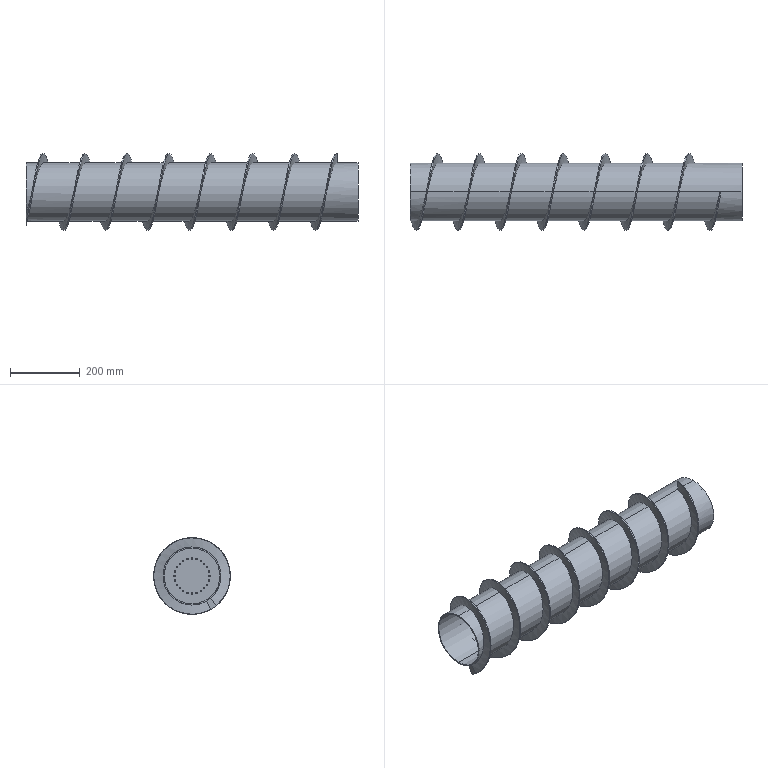Part | SolidWorks | features BaseBody 1 | 1 solid | 74 faces | box 950 x 219.335 x 219.335 mm | volume 1959969 mm3 | cylinder 67 | plane 4 | spline 3 | commonest cylinder face diameters 3.3 x48 166 x17 160 x2